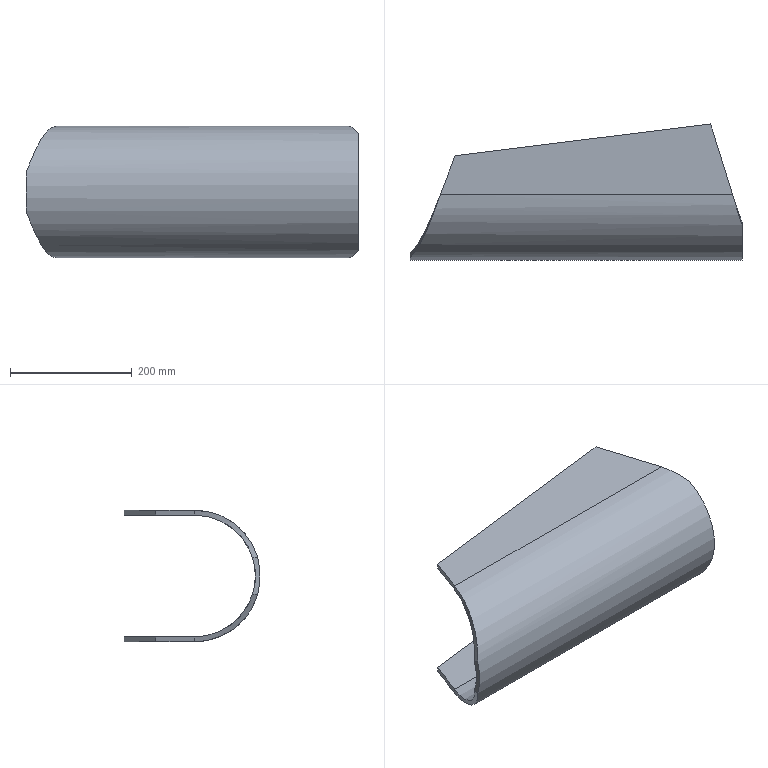Part | SolidWorks | features FlatPattern 1, SM3dBend 1, SMBaseFlange 1, SheetMetal 1 | 1 solid | 18 faces | box 545.7 x 223.987 x 216 mm | volume 2017501 mm3 | plane 12 | spline 4 | cylinder 2 | commonest cylinder face diameters 200 x1 216 x1
STEP:
#1=CARTESIAN_POINT('',(494.2,279.35,208.));
#2=VERTEX_POINT('',#1);
#3=CARTESIAN_POINT('',(530.238,163.363,208.));
#4=VERTEX_POINT('',#3);
#5=CARTESIAN_POINT('',(494.2,279.35,208.));
#6=DIRECTION('',(0.2967,-0.955,0.));
#7=VECTOR('',#6,1000.);
#8=LINE('',#5,#7);
#9=EDGE_CURVE('',#2,#4,#8,.T.);
#10=ORIENTED_EDGE('',*,*,#9,.T.);
#11=CARTESIAN_POINT('',(530.238,163.363,200.));
#12=VERTEX_POINT('',#11);
#13=CARTESIAN_POINT('',(530.238,163.363,208.));
#14=CARTESIAN_POINT('',(530.238,163.363,205.333));
#15=CARTESIAN_POINT('',(530.238,163.363,202.667));
#16=CARTESIAN_POINT('',(530.238,163.363,200.));
#17=B_SPLINE_CURVE_WITH_KNOTS('',3,(#13,#14,#15,#16),.UNSPECIFIED.,.F.,.F.,(4,4),(0.,1.),.UNSPECIFIED.);
#18=EDGE_CURVE('',#4,#12,#17,.T.);
#19=ORIENTED_EDGE('',*,*,#18,.T.);
#20=CARTESIAN_POINT('',(494.2,279.35,200.));
#21=VERTEX_POINT('',#20);
#22=CARTESIAN_POINT('',(494.2,279.35,200.));
#23=DIRECTION('',(0.2967,-0.955,0.));
#24=VECTOR('',#23,1000.);
#25=LINE('',#22,#24);
#26=EDGE_CURVE('',#21,#12,#25,.T.);
#27=ORIENTED_EDGE('',*,*,#26,.F.);
#28=CARTESIAN_POINT('',(494.2,279.35,208.));
#29=DIRECTION('',(0.,0.,-1.));
#30=VECTOR('',#29,1000.);
#31=LINE('',#28,#30);
#32=EDGE_CURVE('',#2,#21,#31,.T.);
#33=ORIENTED_EDGE('',*,*,#32,.F.);
#34=EDGE_LOOP('',(#10,#19,#27,#33));
#35=FACE_OUTER_BOUND('',#34,.T.);
#36=CARTESIAN_POINT('',(494.2,279.35,208.));
#37=DIRECTION('',(0.955,0.2967,0.));
#38=DIRECTION('',(0.2967,-0.955,0.));
#39=AXIS2_PLACEMENT_3D('',#36,#37,#38);
#40=PLANE('',#39);
#41=ADVANCED_FACE('',(#35),#40,.T.);
#42=CARTESIAN_POINT('',(50.045,163.363,200.));
#43=VERTEX_POINT('',#42);
#44=CARTESIAN_POINT('',(74.2,227.3,200.));
#45=VERTEX_POINT('',#44);
#46=CARTESIAN_POINT('',(0.,30.9,200.));
#47=DIRECTION('',(0.3534,0.9355,0.));
#48=VECTOR('',#47,1000.);
#49=LINE('',#46,#48);
#50=EDGE_CURVE('',#43,#45,#49,.T.);
#51=ORIENTED_EDGE('',*,*,#50,.F.);
#52=CARTESIAN_POINT('',(50.045,163.363,208.));
#53=VERTEX_POINT('',#52);
#54=CARTESIAN_POINT('',(50.045,163.363,200.));
#55=CARTESIAN_POINT('',(50.045,163.363,202.667));
#56=CARTESIAN_POINT('',(50.045,163.363,205.333));
#57=CARTESIAN_POINT('',(50.045,163.363,208.));
#58=B_SPLINE_CURVE_WITH_KNOTS('',3,(#54,#55,#56,#57),.UNSPECIFIED.,.F.,.F.,(4,4),(0.,1.),.UNSPECIFIED.);
#59=EDGE_CURVE('',#43,#53,#58,.T.);
#60=ORIENTED_EDGE('',*,*,#59,.T.);
#61=CARTESIAN_POINT('',(74.2,227.3,208.));
#62=VERTEX_POINT('',#61);
#63=CARTESIAN_POINT('',(0.,30.9,208.));
#64=DIRECTION('',(0.3534,0.9355,0.));
#65=VECTOR('',#64,1000.);
#66=LINE('',#63,#65);
#67=EDGE_CURVE('',#53,#62,#66,.T.);
#68=ORIENTED_EDGE('',*,*,#67,.T.);
#69=CARTESIAN_POINT('',(74.2,227.3,208.));
#70=DIRECTION('',(0.,0.,-1.));
#71=VECTOR('',#70,1000.);
#72=LINE('',#69,#71);
#73=EDGE_CURVE('',#62,#45,#72,.T.);
#74=ORIENTED_EDGE('',*,*,#73,.T.);
#75=EDGE_LOOP('',(#51,#60,#68,#74));
#76=FACE_OUTER_BOUND('',#75,.T.);
#77=CARTESIAN_POINT('',(0.,30.9,208.));
#78=DIRECTION('',(-0.9355,0.3534,0.));
#79=DIRECTION('',(0.3534,0.9355,0.));
#80=AXIS2_PLACEMENT_3D('',#77,#78,#79);
#81=PLANE('',#80);
#82=ADVANCED_FACE('',(#76),#81,.T.);
#83=ORIENTED_EDGE('',*,*,#67,.F.);
#84=CARTESIAN_POINT('',(545.7,163.363,208.));
#85=DIRECTION('',(1.,0.,0.));
#86=VECTOR('',#85,1000.);
#87=LINE('',#84,#86);
#88=EDGE_CURVE('',#53,#4,#87,.T.);
#89=ORIENTED_EDGE('',*,*,#88,.T.);
#90=ORIENTED_EDGE('',*,*,#9,.F.);
#91=CARTESIAN_POINT('',(74.2,227.3,208.));
#92=DIRECTION('',(0.9924,0.123,0.));
#93=VECTOR('',#92,1000.);
#94=LINE('',#91,#93);
#95=EDGE_CURVE('',#62,#2,#94,.T.);
#96=ORIENTED_EDGE('',*,*,#95,.F.);
#97=EDGE_LOOP('',(#83,#89,#90,#96));
#98=FACE_OUTER_BOUND('',#97,.T.);
#99=CARTESIAN_POINT('',(545.7,285.732,208.));
#100=DIRECTION('',(0.,0.,1.));
#101=DIRECTION('',(-1.,0.,0.));
#102=AXIS2_PLACEMENT_3D('',#99,#100,#101);
#103=PLANE('',#102);
#104=ADVANCED_FACE('',(#98),#103,.T.);
#105=CARTESIAN_POINT('',(74.2,227.3,200.));
#106=DIRECTION('',(0.9924,0.123,0.));
#107=VECTOR('',#106,1000.);
#108=LINE('',#105,#107);
#109=EDGE_CURVE('',#45,#21,#108,.T.);
#110=ORIENTED_EDGE('',*,*,#109,.F.);
#111=ORIENTED_EDGE('',*,*,#73,.F.);
#112=ORIENTED_EDGE('',*,*,#95,.T.);
#113=ORIENTED_EDGE('',*,*,#32,.T.);
#114=EDGE_LOOP('',(#110,#111,#112,#113));
#115=FACE_OUTER_BOUND('',#114,.T.);
#116=CARTESIAN_POINT('',(74.2,227.3,208.));
#117=DIRECTION('',(-0.123,0.9924,0.));
#118=DIRECTION('',(0.9924,0.123,0.));
#119=AXIS2_PLACEMENT_3D('',#116,#117,#118);
#120=PLANE('',#119);
#121=ADVANCED_FACE('',(#115),#120,.T.);
#122=CARTESIAN_POINT('',(545.7,163.363,200.));
#123=DIRECTION('',(1.,0.,0.));
#124=VECTOR('',#123,1000.);
#125=LINE('',#122,#124);
#126=EDGE_CURVE('',#43,#12,#125,.T.);
#127=ORIENTED_EDGE('',*,*,#126,.F.);
#128=ORIENTED_EDGE('',*,*,#50,.T.);
#129=ORIENTED_EDGE('',*,*,#109,.T.);
#130=ORIENTED_EDGE('',*,*,#26,.T.);
#131=EDGE_LOOP('',(#127,#128,#129,#130));
#132=FACE_OUTER_BOUND('',#131,.T.);
#133=CARTESIAN_POINT('',(545.7,285.732,200.));
#134=DIRECTION('',(0.,0.,1.));
#135=DIRECTION('',(-1.,0.,0.));
#136=AXIS2_PLACEMENT_3D('',#133,#134,#135);
#137=PLANE('',#136);
#138=ADVANCED_FACE('',(#132),#137,.F.);
#139=CARTESIAN_POINT('',(494.2,279.35,0.));
#140=VERTEX_POINT('',#139);
#141=CARTESIAN_POINT('',(74.2,227.3,0.));
#142=VERTEX_POINT('',#141);
#143=CARTESIAN_POINT('',(74.2,227.3,0.));
#144=DIRECTION('',(-0.9924,-0.123,0.));
#145=VECTOR('',#144,1000.);
#146=LINE('',#143,#145);
#147=EDGE_CURVE('',#140,#142,#146,.T.);
#148=ORIENTED_EDGE('',*,*,#147,.F.);
#149=CARTESIAN_POINT('',(494.2,279.35,-8.));
#150=VERTEX_POINT('',#149);
#151=CARTESIAN_POINT('',(494.2,279.35,-8.));
#152=DIRECTION('',(0.,0.,1.));
#153=VECTOR('',#152,1000.);
#154=LINE('',#151,#153);
#155=EDGE_CURVE('',#150,#140,#154,.T.);
#156=ORIENTED_EDGE('',*,*,#155,.F.);
#157=CARTESIAN_POINT('',(74.2,227.3,-8.));
#158=VERTEX_POINT('',#157);
#159=CARTESIAN_POINT('',(74.2,227.3,-8.));
#160=DIRECTION('',(-0.9924,-0.123,0.));
#161=VECTOR('',#160,1000.);
#162=LINE('',#159,#161);
#163=EDGE_CURVE('',#150,#158,#162,.T.);
#164=ORIENTED_EDGE('',*,*,#163,.T.);
#165=CARTESIAN_POINT('',(74.2,227.3,-8.));
#166=DIRECTION('',(0.,0.,1.));
#167=VECTOR('',#166,1000.);
#168=LINE('',#165,#167);
#169=EDGE_CURVE('',#158,#142,#168,.T.);
#170=ORIENTED_EDGE('',*,*,#169,.T.);
#171=EDGE_LOOP('',(#148,#156,#164,#170));
#172=FACE_OUTER_BOUND('',#171,.T.);
#173=CARTESIAN_POINT('',(74.2,227.3,-8.));
#174=DIRECTION('',(-0.123,0.9924,0.));
#175=DIRECTION('',(-0.9924,-0.123,0.));
#176=AXIS2_PLACEMENT_3D('',#173,#174,#175);
#177=PLANE('',#176);
#178=ADVANCED_FACE('',(#172),#177,.T.);
#179=CARTESIAN_POINT('',(50.045,163.363,-8.));
#180=VERTEX_POINT('',#179);
#181=CARTESIAN_POINT('',(530.238,163.363,-8.));
#182=VERTEX_POINT('',#181);
#183=CARTESIAN_POINT('',(545.7,163.363,-8.));
#184=DIRECTION('',(1.,0.,0.));
#185=VECTOR('',#184,1000.);
#186=LINE('',#183,#185);
#187=EDGE_CURVE('',#180,#182,#186,.T.);
#188=ORIENTED_EDGE('',*,*,#187,.F.);
#189=CARTESIAN_POINT('',(0.,30.9,-8.));
#190=DIRECTION('',(-0.3534,-0.9355,0.));
#191=VECTOR('',#190,1000.);
#192=LINE('',#189,#191);
#193=EDGE_CURVE('',#158,#180,#192,.T.);
#194=ORIENTED_EDGE('',*,*,#193,.F.);
#195=ORIENTED_EDGE('',*,*,#163,.F.);
#196=CARTESIAN_POINT('',(494.2,279.35,-8.));
#197=DIRECTION('',(-0.2967,0.955,0.));
#198=VECTOR('',#197,1000.);
#199=LINE('',#196,#198);
#200=EDGE_CURVE('',#182,#150,#199,.T.);
#201=ORIENTED_EDGE('',*,*,#200,.F.);
#202=EDGE_LOOP('',(#188,#194,#195,#201));
#203=FACE_OUTER_BOUND('',#202,.T.);
#204=CARTESIAN_POINT('',(545.7,-285.732,-8.));
#205=DIRECTION('',(0.,0.,-1.));
#206=DIRECTION('',(-1.,0.,0.));
#207=AXIS2_PLACEMENT_3D('',#204,#205,#206);
#208=PLANE('',#207);
#209=ADVANCED_FACE('',(#203),#208,.T.);
#210=CARTESIAN_POINT('',(50.045,163.363,0.));
#211=VERTEX_POINT('',#210);
#212=CARTESIAN_POINT('',(50.045,163.363,0.));
#213=CARTESIAN_POINT('',(50.045,163.363,-8.));
#214=B_SPLINE_CURVE_WITH_KNOTS('',1,(#212,#213),.UNSPECIFIED.,.F.,.F.,(2,2),(0.,1.),.UNSPECIFIED.);
#215=EDGE_CURVE('',#211,#180,#214,.T.);
#216=ORIENTED_EDGE('',*,*,#215,.F.);
#217=CARTESIAN_POINT('',(0.,30.9,0.));
#218=DIRECTION('',(-0.3534,-0.9355,0.));
#219=VECTOR('',#218,1000.);
#220=LINE('',#217,#219);
#221=EDGE_CURVE('',#142,#211,#220,.T.);
#222=ORIENTED_EDGE('',*,*,#221,.F.);
#223=ORIENTED_EDGE('',*,*,#169,.F.);
#224=ORIENTED_EDGE('',*,*,#193,.T.);
#225=EDGE_LOOP('',(#216,#222,#223,#224));
#226=FACE_OUTER_BOUND('',#225,.T.);
#227=CARTESIAN_POINT('',(0.,30.9,-8.));
#228=DIRECTION('',(-0.9355,0.3534,0.));
#229=DIRECTION('',(-0.3534,-0.9355,0.));
#230=AXIS2_PLACEMENT_3D('',#227,#228,#229);
#231=PLANE('',#230);
#232=ADVANCED_FACE('',(#226),#231,.T.);
#233=ORIENTED_EDGE('',*,*,#221,.T.);
#234=CARTESIAN_POINT('',(530.238,163.363,0.));
#235=VERTEX_POINT('',#234);
#236=CARTESIAN_POINT('',(545.7,163.363,0.));
#237=DIRECTION('',(1.,0.,0.));
#238=VECTOR('',#237,1000.);
#239=LINE('',#236,#238);
#240=EDGE_CURVE('',#211,#235,#239,.T.);
#241=ORIENTED_EDGE('',*,*,#240,.T.);
#242=CARTESIAN_POINT('',(494.2,279.35,0.));
#243=DIRECTION('',(-0.2967,0.955,0.));
#244=VECTOR('',#243,1000.);
#245=LINE('',#242,#244);
#246=EDGE_CURVE('',#235,#140,#245,.T.);
#247=ORIENTED_EDGE('',*,*,#246,.T.);
#248=ORIENTED_EDGE('',*,*,#147,.T.);
#249=EDGE_LOOP('',(#233,#241,#247,#248));
#250=FACE_OUTER_BOUND('',#249,.T.);
#251=CARTESIAN_POINT('',(545.7,-285.732,0.));
#252=DIRECTION('',(0.,0.,-1.));
#253=DIRECTION('',(-1.,0.,0.));
#254=AXIS2_PLACEMENT_3D('',#251,#252,#253);
#255=PLANE('',#254);
#256=ADVANCED_FACE('',(#250),#255,.F.);
#257=CARTESIAN_POINT('',(530.238,163.363,-8.));
#258=CARTESIAN_POINT('',(530.238,163.363,0.));
#259=B_SPLINE_CURVE_WITH_KNOTS('',1,(#257,#258),.UNSPECIFIED.,.F.,.F.,(2,2),(0.,1.),.UNSPECIFIED.);
#260=EDGE_CURVE('',#182,#235,#259,.T.);
#261=ORIENTED_EDGE('',*,*,#260,.F.);
#262=ORIENTED_EDGE('',*,*,#200,.T.);
#263=ORIENTED_EDGE('',*,*,#155,.T.);
#264=ORIENTED_EDGE('',*,*,#246,.F.);
#265=EDGE_LOOP('',(#261,#262,#263,#264));
#266=FACE_OUTER_BOUND('',#265,.T.);
#267=CARTESIAN_POINT('',(494.2,279.35,-8.));
#268=DIRECTION('',(0.955,0.2967,0.));
#269=DIRECTION('',(-0.2967,0.955,0.));
#270=AXIS2_PLACEMENT_3D('',#267,#268,#269);
#271=PLANE('',#270);
#272=ADVANCED_FACE('',(#266),#271,.T.);
#273=ORIENTED_EDGE('',*,*,#59,.F.);
#274=CARTESIAN_POINT('',(0.,67.744,129.276));
#275=VERTEX_POINT('',#274);
#276=CARTESIAN_POINT('',(50.045,163.363,200.));
#277=CARTESIAN_POINT('',(45.874,152.748,200.));
#278=CARTESIAN_POINT('',(41.704,142.137,198.296));
#279=CARTESIAN_POINT('',(33.363,121.976,191.65));
#280=CARTESIAN_POINT('',(29.193,112.43,186.71));
#281=CARTESIAN_POINT('',(20.852,95.364,174.086));
#282=CARTESIAN_POINT('',(16.682,87.845,166.406));
#283=CARTESIAN_POINT('',(8.341,75.588,149.074));
#284=CARTESIAN_POINT('',(4.171,70.852,139.426));
#285=CARTESIAN_POINT('',(0.,67.744,129.276));
#286=B_SPLINE_CURVE_WITH_KNOTS('',3,(#276,#277,#278,#279,#280,#281,#282,#283,#284,#285),.UNSPECIFIED.,.F.,.F.,(4,2,2,2,4),(0.,0.25,0.5,0.75,1.),.UNSPECIFIED.);
#287=EDGE_CURVE('',#43,#275,#286,.T.);
#288=ORIENTED_EDGE('',*,*,#287,.T.);
#289=CARTESIAN_POINT('',(0.,60.095,131.618));
#290=VERTEX_POINT('',#289);
#291=CARTESIAN_POINT('',(0.,67.744,129.276));
#292=CARTESIAN_POINT('',(0.,60.095,131.618));
#293=B_SPLINE_CURVE_WITH_KNOTS('',1,(#291,#292),.UNSPECIFIED.,.F.,.F.,(2,2),(0.,1.),.UNSPECIFIED.);
#294=EDGE_CURVE('',#275,#290,#293,.T.);
#295=ORIENTED_EDGE('',*,*,#294,.T.);
#296=CARTESIAN_POINT('',(50.045,163.363,208.));
#297=CARTESIAN_POINT('',(47.959,157.631,208.));
#298=CARTESIAN_POINT('',(45.874,151.9,207.543));
#299=CARTESIAN_POINT('',(41.704,140.582,205.725));
#300=CARTESIAN_POINT('',(39.619,134.995,204.365));
#301=CARTESIAN_POINT('',(35.448,124.108,200.777));
#302=CARTESIAN_POINT('',(33.363,118.808,198.548));
#303=CARTESIAN_POINT('',(29.193,108.628,193.279));
#304=CARTESIAN_POINT('',(27.107,103.748,190.238));
#305=CARTESIAN_POINT('',(22.937,94.532,183.421));
#306=CARTESIAN_POINT('',(20.852,90.196,179.645));
#307=CARTESIAN_POINT('',(16.682,82.177,171.454));
#308=CARTESIAN_POINT('',(14.596,78.494,167.038));
#309=CARTESIAN_POINT('',(10.426,71.875,157.679));
#310=CARTESIAN_POINT('',(8.341,68.939,152.736));
#311=CARTESIAN_POINT('',(4.17,63.888,142.445));
#312=CARTESIAN_POINT('',(2.085,61.773,137.099));
#313=CARTESIAN_POINT('',(0.,60.095,131.618));
#314=B_SPLINE_CURVE_WITH_KNOTS('',3,(#296,#297,#298,#299,#300,#301,#302,#303,#304,#305,#306,#307,#308,#309,#310,#311,#312,#313),.UNSPECIFIED.,.F.,.F.,(4,2,2,2,2,2,2,2,4),(0.,0.125,0.25,0.375,0.5,0.625,0.75,0.875,1.),.UNSPECIFIED.);
#315=EDGE_CURVE('',#53,#290,#314,.T.);
#316=ORIENTED_EDGE('',*,*,#315,.F.);
#317=EDGE_LOOP('',(#273,#288,#295,#316));
#318=FACE_OUTER_BOUND('',#317,.T.);
#319=CARTESIAN_POINT('',(50.045,163.363,208.));
#320=CARTESIAN_POINT('',(45.874,151.899,208.));
#321=CARTESIAN_POINT('',(41.704,140.439,206.16));
#322=CARTESIAN_POINT('',(33.363,118.665,198.982));
#323=CARTESIAN_POINT('',(29.193,108.356,193.646));
#324=CARTESIAN_POINT('',(20.852,89.924,180.013));
#325=CARTESIAN_POINT('',(16.682,81.803,171.718));
#326=CARTESIAN_POINT('',(8.341,68.566,153.));
#327=CARTESIAN_POINT('',(4.171,63.451,142.58));
#328=CARTESIAN_POINT('',(0.,60.095,131.618));
#329=CARTESIAN_POINT('',(50.045,163.363,200.));
#330=CARTESIAN_POINT('',(45.874,152.748,200.));
#331=CARTESIAN_POINT('',(41.704,142.137,198.296));
#332=CARTESIAN_POINT('',(33.363,121.976,191.65));
#333=CARTESIAN_POINT('',(29.193,112.43,186.71));
#334=CARTESIAN_POINT('',(20.852,95.364,174.086));
#335=CARTESIAN_POINT('',(16.682,87.845,166.406));
#336=CARTESIAN_POINT('',(8.341,75.588,149.074));
#337=CARTESIAN_POINT('',(4.171,70.852,139.426));
#338=CARTESIAN_POINT('',(0.,67.744,129.276));
#339=B_SPLINE_SURFACE_WITH_KNOTS('',1,3,((#319,#320,#321,#322,#323,#324,#325,#326,#327,#328),(#329,#330,#331,#332,#333,#334,#335,#336,#337,#338)),.UNSPECIFIED.,.F.,.F.,.F.,(2,2),(4,2,2,2,4),(0.,1.),(0.,0.25,0.5,0.75,1.),.UNSPECIFIED.);
#340=ADVANCED_FACE('',(#318),#339,.T.);
#341=ORIENTED_EDGE('',*,*,#294,.F.);
#342=CARTESIAN_POINT('',(0.,67.744,70.724));
#343=VERTEX_POINT('',#342);
#344=CARTESIAN_POINT('',(0.,163.363,100.));
#345=DIRECTION('',(1.,0.,0.));
#346=DIRECTION('',(0.,0.,1.));
#347=AXIS2_PLACEMENT_3D('',#344,#345,#346);
#348=CIRCLE('',#347,100.);
#349=EDGE_CURVE('',#275,#343,#348,.T.);
#350=ORIENTED_EDGE('',*,*,#349,.T.);
#351=CARTESIAN_POINT('',(0.,60.095,68.382));
#352=VERTEX_POINT('',#351);
#353=CARTESIAN_POINT('',(0.,67.744,70.724));
#354=CARTESIAN_POINT('',(0.,65.194,69.943));
#355=CARTESIAN_POINT('',(0.,62.645,69.162));
#356=CARTESIAN_POINT('',(0.,60.095,68.382));
#357=B_SPLINE_CURVE_WITH_KNOTS('',3,(#353,#354,#355,#356),.UNSPECIFIED.,.F.,.F.,(4,4),(0.,1.),.UNSPECIFIED.);
#358=EDGE_CURVE('',#343,#352,#357,.T.);
#359=ORIENTED_EDGE('',*,*,#358,.T.);
#360=CARTESIAN_POINT('',(0.,163.363,100.));
#361=DIRECTION('',(1.,0.,0.));
#362=DIRECTION('',(0.,0.,1.));
#363=AXIS2_PLACEMENT_3D('',#360,#361,#362);
#364=CIRCLE('',#363,108.);
#365=EDGE_CURVE('',#290,#352,#364,.T.);
#366=ORIENTED_EDGE('',*,*,#365,.F.);
#367=EDGE_LOOP('',(#341,#350,#359,#366));
#368=FACE_OUTER_BOUND('',#367,.T.);
#369=CARTESIAN_POINT('',(0.,163.363,100.));
#370=DIRECTION('',(-1.,0.,0.));
#371=DIRECTION('',(0.,0.,1.));
#372=AXIS2_PLACEMENT_3D('',#369,#370,#371);
#373=PLANE('',#372);
#374=ADVANCED_FACE('',(#368),#373,.T.);
#375=ORIENTED_EDGE('',*,*,#358,.F.);
#376=CARTESIAN_POINT('',(0.,67.744,70.724));
#377=CARTESIAN_POINT('',(4.171,70.852,60.574));
#378=CARTESIAN_POINT('',(8.341,75.588,50.926));
#379=CARTESIAN_POINT('',(16.682,87.845,33.594));
#380=CARTESIAN_POINT('',(20.852,95.364,25.914));
#381=CARTESIAN_POINT('',(29.193,112.43,13.29));
#382=CARTESIAN_POINT('',(33.363,121.976,8.35));
#383=CARTESIAN_POINT('',(41.704,142.137,1.704));
#384=CARTESIAN_POINT('',(45.874,152.748,0.));
#385=CARTESIAN_POINT('',(50.045,163.363,0.));
#386=B_SPLINE_CURVE_WITH_KNOTS('',3,(#376,#377,#378,#379,#380,#381,#382,#383,#384,#385),.UNSPECIFIED.,.F.,.F.,(4,2,2,2,4),(0.,0.25,0.5,0.75,1.),.UNSPECIFIED.);
#387=EDGE_CURVE('',#343,#211,#386,.T.);
#388=ORIENTED_EDGE('',*,*,#387,.T.);
#389=ORIENTED_EDGE('',*,*,#215,.T.);
#390=CARTESIAN_POINT('',(0.,60.095,68.382));
#391=CARTESIAN_POINT('',(2.085,61.773,62.901));
#392=CARTESIAN_POINT('',(4.17,63.888,57.555));
#393=CARTESIAN_POINT('',(8.341,68.939,47.264));
#394=CARTESIAN_POINT('',(10.426,71.875,42.321));
#395=CARTESIAN_POINT('',(14.596,78.494,32.962));
#396=CARTESIAN_POINT('',(16.682,82.177,28.546));
#397=CARTESIAN_POINT('',(20.852,90.196,20.355));
#398=CARTESIAN_POINT('',(22.937,94.532,16.579));
#399=CARTESIAN_POINT('',(27.107,103.748,9.762));
#400=CARTESIAN_POINT('',(29.193,108.628,6.721));
#401=CARTESIAN_POINT('',(33.363,118.808,1.452));
#402=CARTESIAN_POINT('',(35.448,124.108,-0.7766));
#403=CARTESIAN_POINT('',(39.619,134.995,-4.365));
#404=CARTESIAN_POINT('',(41.704,140.582,-5.725));
#405=CARTESIAN_POINT('',(45.874,151.9,-7.543));
#406=CARTESIAN_POINT('',(47.959,157.631,-8.));
#407=CARTESIAN_POINT('',(50.045,163.363,-8.));
#408=B_SPLINE_CURVE_WITH_KNOTS('',3,(#390,#391,#392,#393,#394,#395,#396,#397,#398,#399,#400,#401,#402,#403,#404,#405,#406,#407),.UNSPECIFIED.,.F.,.F.,(4,2,2,2,2,2,2,2,4),(0.,0.125,0.25,0.375,0.5,0.625,0.75,0.875,1.),.UNSPECIFIED.);
#409=EDGE_CURVE('',#352,#180,#408,.T.);
#410=ORIENTED_EDGE('',*,*,#409,.F.);
#411=EDGE_LOOP('',(#375,#388,#389,#410));
#412=FACE_OUTER_BOUND('',#411,.T.);
#413=CARTESIAN_POINT('',(0.,60.095,68.382));
#414=CARTESIAN_POINT('',(4.171,63.451,57.42));
#415=CARTESIAN_POINT('',(8.341,68.566,47.));
#416=CARTESIAN_POINT('',(16.682,81.803,28.282));
#417=CARTESIAN_POINT('',(20.852,89.924,19.987));
#418=CARTESIAN_POINT('',(29.193,108.356,6.354));
#419=CARTESIAN_POINT('',(33.363,118.665,1.018));
#420=CARTESIAN_POINT('',(41.704,140.439,-6.16));
#421=CARTESIAN_POINT('',(45.874,151.899,-8.));
#422=CARTESIAN_POINT('',(50.045,163.363,-8.));
#423=CARTESIAN_POINT('',(0.,67.744,70.724));
#424=CARTESIAN_POINT('',(4.171,70.852,60.574));
#425=CARTESIAN_POINT('',(8.341,75.588,50.926));
#426=CARTESIAN_POINT('',(16.682,87.845,33.594));
#427=CARTESIAN_POINT('',(20.852,95.364,25.914));
#428=CARTESIAN_POINT('',(29.193,112.43,13.29));
#429=CARTESIAN_POINT('',(33.363,121.976,8.35));
#430=CARTESIAN_POINT('',(41.704,142.137,1.704));
#431=CARTESIAN_POINT('',(45.874,152.748,0.));
#432=CARTESIAN_POINT('',(50.045,163.363,0.));
#433=B_SPLINE_SURFACE_WITH_KNOTS('',1,3,((#413,#414,#415,#416,#417,#418,#419,#420,#421,#422),(#423,#424,#425,#426,#427,#428,#429,#430,#431,#432)),.UNSPECIFIED.,.F.,.F.,.F.,(2,2),(4,2,2,2,4),(0.,1.),(0.,0.25,0.5,0.75,1.),.UNSPECIFIED.);
#434=ADVANCED_FACE('',(#412),#433,.T.);
#435=ORIENTED_EDGE('',*,*,#260,.T.);
#436=CARTESIAN_POINT('',(545.7,117.319,11.231));
#437=VERTEX_POINT('',#436);
#438=CARTESIAN_POINT('',(530.238,163.363,0.));
#439=CARTESIAN_POINT('',(532.815,155.388,0.));
#440=CARTESIAN_POINT('',(535.392,147.414,0.9585));
#441=CARTESIAN_POINT('',(540.546,131.918,4.738));
#442=CARTESIAN_POINT('',(543.123,124.398,7.559));
#443=CARTESIAN_POINT('',(545.7,117.319,11.231));
#444=B_SPLINE_CURVE_WITH_KNOTS('',3,(#438,#439,#440,#441,#442,#443),.UNSPECIFIED.,.F.,.F.,(4,2,4),(0.,0.5,1.),.UNSPECIFIED.);
#445=EDGE_CURVE('',#235,#437,#444,.T.);
#446=ORIENTED_EDGE('',*,*,#445,.T.);
#447=CARTESIAN_POINT('',(545.7,113.636,4.129));
#448=VERTEX_POINT('',#447);
#449=CARTESIAN_POINT('',(545.7,117.319,11.231));
#450=CARTESIAN_POINT('',(545.7,113.636,4.129));
#451=B_SPLINE_CURVE_WITH_KNOTS('',1,(#449,#450),.UNSPECIFIED.,.F.,.F.,(2,2),(0.,1.),.UNSPECIFIED.);
#452=EDGE_CURVE('',#437,#448,#451,.T.);
#453=ORIENTED_EDGE('',*,*,#452,.T.);
#454=CARTESIAN_POINT('',(530.238,163.363,-8.));
#455=CARTESIAN_POINT('',(532.815,154.75,-8.));
#456=CARTESIAN_POINT('',(535.392,146.138,-6.965));
#457=CARTESIAN_POINT('',(540.546,129.403,-2.883));
#458=CARTESIAN_POINT('',(543.123,121.281,0.1636));
#459=CARTESIAN_POINT('',(545.7,113.636,4.129));
#460=B_SPLINE_CURVE_WITH_KNOTS('',3,(#454,#455,#456,#457,#458,#459),.UNSPECIFIED.,.F.,.F.,(4,2,4),(0.,0.5,1.),.UNSPECIFIED.);
#461=EDGE_CURVE('',#182,#448,#460,.T.);
#462=ORIENTED_EDGE('',*,*,#461,.F.);
#463=EDGE_LOOP('',(#435,#446,#453,#462));
#464=FACE_OUTER_BOUND('',#463,.T.);
#465=CARTESIAN_POINT('',(530.238,163.363,-8.));
#466=CARTESIAN_POINT('',(532.815,154.75,-8.));
#467=CARTESIAN_POINT('',(535.392,146.138,-6.965));
#468=CARTESIAN_POINT('',(540.546,129.403,-2.883));
#469=CARTESIAN_POINT('',(543.123,121.281,0.1635));
#470=CARTESIAN_POINT('',(545.7,113.636,4.129));
#471=CARTESIAN_POINT('',(530.238,163.363,0.));
#472=CARTESIAN_POINT('',(532.815,155.388,0.));
#473=CARTESIAN_POINT('',(535.392,147.414,0.9585));
#474=CARTESIAN_POINT('',(540.546,131.918,4.738));
#475=CARTESIAN_POINT('',(543.123,124.398,7.559));
#476=CARTESIAN_POINT('',(545.7,117.319,11.231));
#477=B_SPLINE_SURFACE_WITH_KNOTS('',1,3,((#465,#466,#467,#468,#469,#470),(#471,#472,#473,#474,#475,#476)),.UNSPECIFIED.,.F.,.F.,.F.,(2,2),(4,2,4),(0.,1.),(0.,0.5,1.),.UNSPECIFIED.);
#478=ADVANCED_FACE('',(#464),#477,.T.);
#479=ORIENTED_EDGE('',*,*,#452,.F.);
#480=CARTESIAN_POINT('',(545.7,117.319,188.769));
#481=VERTEX_POINT('',#480);
#482=CARTESIAN_POINT('',(545.7,163.363,100.));
#483=DIRECTION('',(-1.,0.,0.));
#484=DIRECTION('',(0.,0.,1.));
#485=AXIS2_PLACEMENT_3D('',#482,#483,#484);
#486=CIRCLE('',#485,100.);
#487=EDGE_CURVE('',#437,#481,#486,.T.);
#488=ORIENTED_EDGE('',*,*,#487,.T.);
#489=CARTESIAN_POINT('',(545.7,113.636,195.871));
#490=VERTEX_POINT('',#489);
#491=CARTESIAN_POINT('',(545.7,117.319,188.769));
#492=CARTESIAN_POINT('',(545.7,116.091,191.136));
#493=CARTESIAN_POINT('',(545.7,114.863,193.504));
#494=CARTESIAN_POINT('',(545.7,113.636,195.871));
#495=B_SPLINE_CURVE_WITH_KNOTS('',3,(#491,#492,#493,#494),.UNSPECIFIED.,.F.,.F.,(4,4),(0.,1.),.UNSPECIFIED.);
#496=EDGE_CURVE('',#481,#490,#495,.T.);
#497=ORIENTED_EDGE('',*,*,#496,.T.);
#498=CARTESIAN_POINT('',(545.7,163.363,100.));
#499=DIRECTION('',(-1.,0.,0.));
#500=DIRECTION('',(0.,0.,-1.));
#501=AXIS2_PLACEMENT_3D('',#498,#499,#500);
#502=CIRCLE('',#501,108.);
#503=EDGE_CURVE('',#448,#490,#502,.T.);
#504=ORIENTED_EDGE('',*,*,#503,.F.);
#505=EDGE_LOOP('',(#479,#488,#497,#504));
#506=FACE_OUTER_BOUND('',#505,.T.);
#507=CARTESIAN_POINT('',(545.7,163.363,100.));
#508=DIRECTION('',(1.,0.,0.));
#509=DIRECTION('',(0.,0.,-1.));
#510=AXIS2_PLACEMENT_3D('',#507,#508,#509);
#511=PLANE('',#510);
#512=ADVANCED_FACE('',(#506),#511,.T.);
#513=ORIENTED_EDGE('',*,*,#503,.T.);
#514=CARTESIAN_POINT('',(545.7,113.636,195.871));
#515=CARTESIAN_POINT('',(543.123,121.281,199.836));
#516=CARTESIAN_POINT('',(540.546,129.403,202.883));
#517=CARTESIAN_POINT('',(535.392,146.138,206.965));
#518=CARTESIAN_POINT('',(532.815,154.75,208.));
#519=CARTESIAN_POINT('',(530.238,163.363,208.));
#520=B_SPLINE_CURVE_WITH_KNOTS('',3,(#514,#515,#516,#517,#518,#519),.UNSPECIFIED.,.F.,.F.,(4,2,4),(0.,0.5,1.),.UNSPECIFIED.);
#521=EDGE_CURVE('',#490,#4,#520,.T.);
#522=ORIENTED_EDGE('',*,*,#521,.T.);
#523=ORIENTED_EDGE('',*,*,#88,.F.);
#524=ORIENTED_EDGE('',*,*,#315,.T.);
#525=ORIENTED_EDGE('',*,*,#365,.T.);
#526=ORIENTED_EDGE('',*,*,#409,.T.);
#527=ORIENTED_EDGE('',*,*,#187,.T.);
#528=ORIENTED_EDGE('',*,*,#461,.T.);
#529=EDGE_LOOP('',(#513,#522,#523,#524,#525,#526,#527,#528));
#530=FACE_OUTER_BOUND('',#529,.T.);
#531=CARTESIAN_POINT('',(926.225,163.363,100.));
#532=DIRECTION('',(-1.,0.,0.));
#533=DIRECTION('',(0.,0.,1.));
#534=AXIS2_PLACEMENT_3D('',#531,#532,#533);
#535=CYLINDRICAL_SURFACE('',#534,108.);
#536=ADVANCED_FACE('',(#530),#535,.T.);
#537=CARTESIAN_POINT('',(545.7,117.319,188.769));
#538=CARTESIAN_POINT('',(543.123,124.398,192.441));
#539=CARTESIAN_POINT('',(540.546,131.918,195.262));
#540=CARTESIAN_POINT('',(535.392,147.414,199.042));
#541=CARTESIAN_POINT('',(532.815,155.388,200.));
#542=CARTESIAN_POINT('',(530.238,163.363,200.));
#543=B_SPLINE_CURVE_WITH_KNOTS('',3,(#537,#538,#539,#540,#541,#542),.UNSPECIFIED.,.F.,.F.,(4,2,4),(0.,0.5,1.),.UNSPECIFIED.);
#544=EDGE_CURVE('',#481,#12,#543,.T.);
#545=ORIENTED_EDGE('',*,*,#544,.T.);
#546=ORIENTED_EDGE('',*,*,#18,.F.);
#547=ORIENTED_EDGE('',*,*,#521,.F.);
#548=ORIENTED_EDGE('',*,*,#496,.F.);
#549=EDGE_LOOP('',(#545,#546,#547,#548));
#550=FACE_OUTER_BOUND('',#549,.T.);
#551=CARTESIAN_POINT('',(545.7,113.636,195.871));
#552=CARTESIAN_POINT('',(543.123,121.281,199.836));
#553=CARTESIAN_POINT('',(540.546,129.403,202.883));
#554=CARTESIAN_POINT('',(535.392,146.138,206.965));
#555=CARTESIAN_POINT('',(532.815,154.75,208.));
#556=CARTESIAN_POINT('',(530.238,163.363,208.));
#557=CARTESIAN_POINT('',(545.7,117.319,188.769));
#558=CARTESIAN_POINT('',(543.123,124.398,192.441));
#559=CARTESIAN_POINT('',(540.546,131.918,195.262));
#560=CARTESIAN_POINT('',(535.392,147.414,199.042));
#561=CARTESIAN_POINT('',(532.815,155.388,200.));
#562=CARTESIAN_POINT('',(530.238,163.363,200.));
#563=B_SPLINE_SURFACE_WITH_KNOTS('',1,3,((#551,#552,#553,#554,#555,#556),(#557,#558,#559,#560,#561,#562)),.UNSPECIFIED.,.F.,.F.,.F.,(2,2),(4,2,4),(0.,1.),(0.,0.5,1.),.UNSPECIFIED.);
#564=ADVANCED_FACE('',(#550),#563,.T.);
#565=ORIENTED_EDGE('',*,*,#487,.F.);
#566=ORIENTED_EDGE('',*,*,#445,.F.);
#567=ORIENTED_EDGE('',*,*,#240,.F.);
#568=ORIENTED_EDGE('',*,*,#387,.F.);
#569=ORIENTED_EDGE('',*,*,#349,.F.);
#570=ORIENTED_EDGE('',*,*,#287,.F.);
#571=ORIENTED_EDGE('',*,*,#126,.T.);
#572=ORIENTED_EDGE('',*,*,#544,.F.);
#573=EDGE_LOOP('',(#565,#566,#567,#568,#569,#570,#571,#572));
#574=FACE_OUTER_BOUND('',#573,.T.);
#575=CARTESIAN_POINT('',(926.225,163.363,100.));
#576=DIRECTION('',(-1.,0.,0.));
#577=DIRECTION('',(0.,0.,1.));
#578=AXIS2_PLACEMENT_3D('',#575,#576,#577);
#579=CYLINDRICAL_SURFACE('',#578,100.);
#580=ADVANCED_FACE('',(#574),#579,.F.);
#581=CLOSED_SHELL('',(#41,#82,#104,#121,#138,#178,#209,#232,#256,#272,#340,#374,#434,#478,#512,#536,#564,#580));
#582=MANIFOLD_SOLID_BREP('',#581);
#583=CARTESIAN_POINT('',(0.,0.,0.));
#584=DIRECTION('',(0.,0.,1.));
#585=DIRECTION('',(1.,0.,0.));
#586=AXIS2_PLACEMENT_3D('',#583,#584,#585);
#587=(LENGTH_UNIT()NAMED_UNIT(*)SI_UNIT(.MILLI.,.METRE.));
#588=UNCERTAINTY_MEASURE_WITH_UNIT(LENGTH_MEASURE(0.00001),#587,'','');
#589=(NAMED_UNIT(*)PLANE_ANGLE_UNIT()SI_UNIT($,.RADIAN.));
#590=(NAMED_UNIT(*)SI_UNIT($,.STERADIAN.)SOLID_ANGLE_UNIT());
#591=(GEOMETRIC_REPRESENTATION_CONTEXT(3)GLOBAL_UNCERTAINTY_ASSIGNED_CONTEXT((#588))GLOBAL_UNIT_ASSIGNED_CONTEXT((#587,#589,#590))REPRESENTATION_CONTEXT('',''));
#592=ADVANCED_BREP_SHAPE_REPRESENTATION('',(#582,#586),#591);